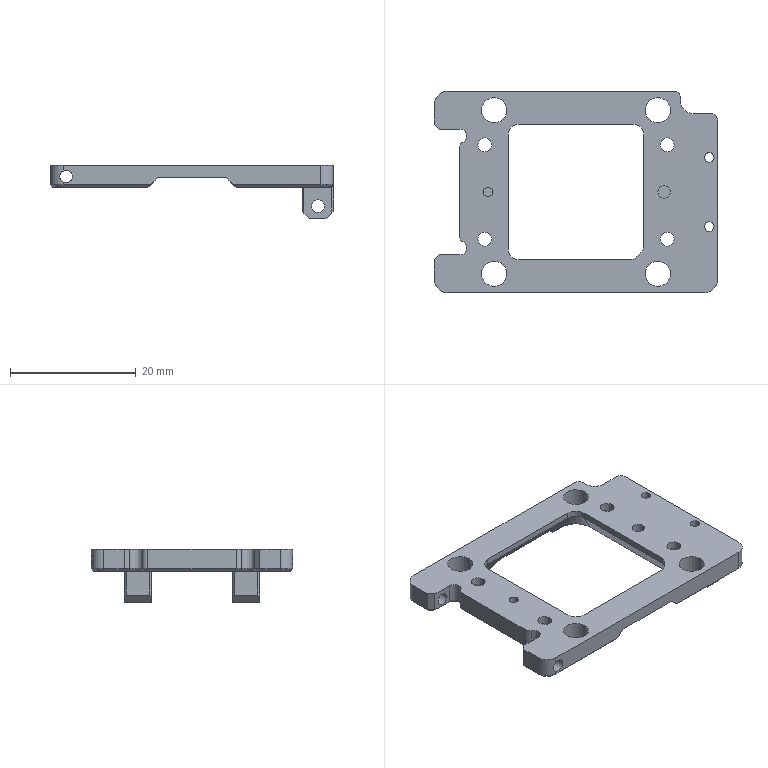NC program | NX | posted with a generic post | part box 45 x 32 x 8.5 mm
Lines 1818 to 2983 of 2983:
(ZLEVEL_PROFILE_1 , TOOL : D3R0.5)
N3592 T07 M6
N3594 G54
N3596 G17 G0 G90 X6.039 Y-10.352 B0. C0. S9500 M3
N3598 G43 Z30. H7
N3600 Z-3.587
N3602 G94 G1 Z-5.087 F1000.
N3604 X6.275 Y-10.756
N3606 G3 X6.536 Y-10.905 R0.3
N3608 G1 X8.847 Y-10.89 F2500.
N3610 G3 X9.951 Y-10.624 R2.492
N3612 X10.883 Y-9.005 R2.038
N3614 G1 X10.892 Y-8.762
N3616 X10.905 Y-5.354
N3618 X10.903 Y7.058
N3620 X10.89 Y8.886
N3622 G3 X10.466 Y10.153 R2.149
N3624 X9.005 Y10.883 R1.989
N3626 G1 X8.762 Y10.891
N3628 X6.571 Y10.904
N3630 X6.536 Y10.906
N3632 X6.444 Y10.858 Z-5.173
N3634 X6.571 Y10.854
N3636 X8.762 Y10.847
N3638 X9.005 Y10.839
N3640 G2 X10.763 Y9.483 R1.865
N3642 X10.848 Y8.88 R2.239
N3644 G1 X10.854 Y7.058
N3646 Y-7.058
N3648 X10.847 Y-8.762
N3650 G2 X10.827 Y-9.156 R3.694
N3652 X9.979 Y-10.559 R1.937
N3654 X8.881 Y-10.848 R2.251
N3656 G1 X6.571 Y-10.853
N3658 X6.444 Y-10.857
N3660 X6.351 Y-10.804 Z-5.26
N3662 X6.99 Y-10.805
N3664 X9.
N3666 G3 X10.045 Y-10.466 R2.012
N3668 X10.805 Y-9. R1.898
N3670 G1 Y9.
N3672 G3 X9. Y10.805 R1.841
N3674 G1 X6.99
N3676 X6.352
N3678 X6.26 Y10.757 Z-5.346
N3680 X6.328 Y10.754
N3682 X6.904 Y10.755
N3684 X9.
N3686 G2 X10.755 Y9. R1.755
N3688 G1 Y-9.
N3690 G2 X9. Y-10.755 R1.755
N3692 G1 X6.904
N3694 X6.328 Y-10.753
N3696 X6.259 Y-10.757
N3698 X6.167 Y-10.705 Z-5.433
N3700 X6.817
N3702 X9.
N3704 G3 X10.705 Y-9. R1.705
N3706 G1 Y9.
N3708 G3 X9. Y10.705 R1.705
N3710 G1 X6.817
N3712 X6.167 Y10.706
N3714 X6.075 Y10.655 Z-5.52
N3716 X6.73
N3718 X9.
N3720 G2 X10.655 Y9. R1.655
N3722 G1 Y-9.
N3724 G2 X9. Y-10.655 R1.655
N3726 G1 X6.73
N3728 X6.075
N3730 X5.983 Y-10.609 Z-5.606
N3732 X6.085 Y-10.604
N3734 X6.644 Y-10.605
N3736 X9.
N3738 G3 X10.605 Y-9. R1.605
N3740 G1 Y9.
N3742 G3 X9. Y10.605 R1.605
N3744 G1 X6.644
N3746 X6.085 Y10.604
N3748 X5.983 Y10.609
N3750 X5.891 Y10.558 Z-5.693
N3752 X6.557 Y10.555
N3754 X9.
N3756 G2 X10.555 Y9. R1.555
N3758 G1 Y-9.
N3760 G2 X9. Y-10.555 R1.555
N3762 G1 X6.557
N3764 X5.891 Y-10.558
N3766 X5.798 Y-10.507 Z-5.779
N3768 X5.841 Y-10.504
N3770 X6.471 Y-10.505
N3772 X9.
N3774 G3 X10.505 Y-9. R1.505
N3776 G1 Y9.
N3778 G3 X9. Y10.505 R1.505
N3780 G1 X6.471
N3782 X5.841
N3784 X5.798 Y10.507
N3786 X5.706 Y10.457 Z-5.866
N3788 X6.384 Y10.455
N3790 X9.
N3792 G2 X10.455 Y9. R1.455
N3794 G1 Y-9.
N3796 G2 X9. Y-10.455 R1.455
N3798 G1 X6.384
N3800 X5.841
N3802 X5.706 Y-10.457
N3804 X5.613 Y-10.405 Z-5.953
N3806 X6.297
N3808 X9.
N3810 G3 X10.405 Y-9. R1.405
N3812 G1 Y9.
N3814 G3 X9. Y10.405 R1.405
N3816 G1 X6.297
N3818 X5.613
N3820 X5.521 Y10.36 Z-6.039
N3822 X5.598 Y10.355
N3824 X6.211
N3826 X9.
N3828 G2 X10.355 Y9. R1.355
N3830 G1 Y-9.
N3832 G2 X9. Y-10.355 R1.355
N3834 G1 X6.211
N3836 X5.598
N3838 X5.521 Y-10.359
N3840 G2 X5.252 Y-10.226 R0.3
N3842 G1 X4.984 Y-9.822
N3844 Z-4.539
N3846 G0 Z30.
N3848 X4.93 Y-9.757
N3850 Z-4.626
N3852 G1 Z-6.126 F1000.
N3854 X5.168 Y-10.161
N3856 G3 X5.428 Y-10.309 R0.3
N3858 G1 X6.124 Y-10.305 F2500.
N3860 X9.
N3862 G3 X10.305 Y-9. R1.305
N3864 G1 Y9.
N3866 G3 X9. Y10.305 R1.305
N3868 G1 X6.124
N3870 X5.428 Y10.309
N3872 X5.336 Y10.256 Z-6.212
N3874 X6.038 Y10.255
N3876 X9.
N3878 G2 X10.255 Y9. R1.255
N3880 G1 Y-9.
N3882 G2 X9. Y-10.255 R1.255
N3884 G1 X6.038
N3886 X5.336 Y-10.256
N3888 X5.219 Y-10.257 Z-6.218
N3890 X5.102 Y-10.258 Z-6.223
N3892 X4.985 Y-10.254 Z-6.229
N3894 X4.868 Y-10.248 Z-6.234
N3896 X4.751 Y-10.245 Z-6.239
N3898 X4.634 Y-10.24 Z-6.245
N3900 X4.516 Y-10.236 Z-6.25
N3902 X4.399 Y-10.232 Z-6.256
N3904 X4.282 Y-10.229 Z-6.261
N3906 X4.165 Y-10.225 Z-6.267
N3908 X4.048 Y-10.221 Z-6.272
N3910 X3.931 Y-10.218 Z-6.277
N3912 X3.814 Y-10.214 Z-6.283
N3914 X3.697 Y-10.211 Z-6.288
N3916 X3.58 Y-10.208 Z-6.294
N3918 X3.463 Y-10.205 Z-6.299
N3920 X5.951
N3922 X9.
N3924 G3 X10.205 Y-9. R1.205
N3926 G1 Y9.
N3928 G3 X9. Y10.205 R1.205
N3930 G1 X5.951
N3932 X3.497
N3934 G3 X3.237 Y10.055 R0.3
N3936 G1 X2.978 Y9.605
N3938 Z-4.799
N3940 G0 Z30.
N3942 X-6.039 Y10.352
N3944 Z-3.587
N3946 G1 Z-5.087 F1000.
N3948 X-6.275 Y10.756
N3950 G3 X-6.536 Y10.905 R0.3
N3952 G1 X-8.762 Y10.89 F2500.
N3954 X-9.005 Y10.882
N3956 G3 X-10.466 Y10.153 R1.983
N3958 X-10.892 Y8.88 R2.18
N3960 G1 X-10.903 Y7.788
N3962 Y-6.815
N3964 X-10.893 Y-8.114
N3966 G3 X-10.827 Y-8.762 R3.463
N3968 X-10.311 Y-9.735 R2.099
N3970 G1 X-9.829 Y-10.222
N3972 X-9.697 Y-10.342
N3974 G3 X-8.657 Y-10.844 R1.994
N3976 X-8.275 Y-10.891 R6.142
N3978 G1 X-6.536 Y-10.906
N3980 X-6.444 Y-10.858 Z-5.173
N3982 X-6.571 Y-10.853
N3984 X-8.275 Y-10.847
N3986 G2 X-9.249 Y-10.609 R2.255
N3988 X-10.008 Y-9.979 R3.046
N3990 X-10.609 Y-9.249 R2.964
N3992 X-10.847 Y-8.275 R2.214
N3994 G1 X-10.854 Y-6.815
N3996 X-10.855 Y4.381
N3998 X-10.848 Y8.762
N4000 X-10.84 Y9.005
N4002 G2 X-9.005 Y10.841 R1.879
N4004 G1 X-8.762 Y10.848
N4006 X-6.571 Y10.853
N4008 X-6.444 Y10.857
N4010 X-6.352 Y10.804 Z-5.26
N4012 X-6.99 Y10.805
N4014 X-9.
N4016 G3 X-10.805 Y9. R1.841
N4018 G1 Y-8.275
N4020 G3 X-10.709 Y-8.929 R2.675
N4022 X-10.222 Y-9.709 R2.104
N4024 G1 X-9.709 Y-10.222
N4026 G3 X-8.929 Y-10.709 R2.066
N4028 X-8.275 Y-10.805 R2.735
N4030 G1 X-6.99
N4032 X-6.352
N4034 X-6.259 Y-10.757 Z-5.346
N4036 X-6.328 Y-10.754
N4038 X-6.904 Y-10.755
N4040 X-8.379
N4042 G2 X-9.619 Y-10.241 R1.755
N4044 G1 X-10.241 Y-9.619
N4046 G2 X-10.755 Y-8.379 R1.755
N4048 G1 Y9.
N4050 G2 X-9. Y10.755 R1.755
N4052 G1 X-6.904
N4054 X-6.328 Y10.753
N4056 X-6.26 Y10.757
N4058 X-6.167 Y10.705 Z-5.433
N4060 X-6.817
N4062 X-9.
N4064 G3 X-10.705 Y9. R1.705
N4066 G1 Y-8.379
N4068 G3 X-10.205 Y-9.584 R1.705
N4070 G1 X-9.584 Y-10.205
N4072 G3 X-8.379 Y-10.705 R1.705
N4074 G1 X-6.817
N4076 X-6.167
N4078 X-6.075 Y-10.655 Z-5.52
N4080 X-6.73
N4082 X-8.379
N4084 G2 X-9.549 Y-10.17 R1.655
N4086 G1 X-10.17 Y-9.549
N4088 G2 X-10.655 Y-8.379 R1.655
N4090 G1 Y9.
N4092 G2 X-9. Y10.655 R1.655
N4094 G1 X-6.73
N4096 X-6.075
N4098 X-5.983 Y10.609 Z-5.606
N4100 X-6.085 Y10.604
N4102 X-6.644 Y10.605
N4104 X-9.
N4106 G3 X-10.605 Y9. R1.605
N4108 G1 Y-8.379
N4110 G3 X-10.135 Y-9.513 R1.605
N4112 G1 X-9.513 Y-10.135
N4114 G3 X-8.379 Y-10.605 R1.605
N4116 G1 X-6.644
N4118 X-6.085 Y-10.604
N4120 X-5.983 Y-10.609
N4122 X-5.891 Y-10.558 Z-5.693
N4124 X-6.557 Y-10.555
N4126 X-8.379
N4128 G2 X-9.478 Y-10.099 R1.555
N4130 G1 X-10.099 Y-9.478
N4132 G2 X-10.555 Y-8.379 R1.555
N4134 G1 Y9.
N4136 G2 X-9. Y10.555 R1.555
N4138 G1 X-6.557
N4140 X-5.891 Y10.558
N4142 X-5.799 Y10.507 Z-5.779
N4144 X-5.841 Y10.505
N4146 X-6.471
N4148 X-9.
N4150 G3 X-10.505 Y9. R1.505
N4152 G1 Y-8.379
N4154 G3 X-10.064 Y-9.443 R1.505
N4156 G1 X-9.443 Y-10.064
N4158 G3 X-8.379 Y-10.505 R1.505
N4160 G1 X-6.471
N4162 X-5.841
N4164 X-5.798 Y-10.507
N4166 X-5.706 Y-10.457 Z-5.866
N4168 X-5.841 Y-10.455
N4170 X-6.384
N4172 X-8.379
N4174 G2 X-9.407 Y-10.029 R1.455
N4176 G1 X-10.029 Y-9.407
N4178 G2 X-10.455 Y-8.379 R1.455
N4180 G1 Y9.
N4182 G2 X-9. Y10.455 R1.455
N4184 G1 X-6.384
N4186 X-5.841
N4188 X-5.706 Y10.457
N4190 X-5.613 Y10.405 Z-5.953
N4192 X-6.297
N4194 X-9.
N4196 G3 X-10.405 Y9. R1.405
N4198 G1 Y-8.379
N4200 G3 X-9.993 Y-9.372 R1.405
N4202 G1 X-9.372 Y-9.993
N4204 G3 X-8.379 Y-10.405 R1.405
N4206 G1 X-6.297
N4208 X-5.613
N4210 X-5.521 Y-10.359 Z-6.039
N4212 X-5.598 Y-10.355
N4214 X-6.211
N4216 X-8.379
N4218 G2 X-9.337 Y-9.958 R1.355
N4220 G1 X-9.958 Y-9.337
N4222 G2 X-10.355 Y-8.379 R1.355
N4224 G1 Y9.
N4226 G2 X-9. Y10.355 R1.355
N4228 G1 X-6.211
N4230 X-5.598
N4232 X-5.521 Y10.359
N4234 G2 X-5.252 Y10.226 R0.3
N4236 G1 X-4.984 Y9.822
N4238 Z-4.539
N4240 G0 Z30.
N4242 X-4.93 Y9.757
N4244 Z-4.626
N4246 G1 Z-6.126 F1000.
N4248 X-5.167 Y10.161
N4250 G3 X-5.428 Y10.309 R0.3
N4252 G1 X-6.124 Y10.305 F2500.
N4254 X-9.
N4256 G3 X-10.305 Y9. R1.305
N4258 G1 Y-8.379
N4260 G3 X-9.923 Y-9.301 R1.305
N4262 G1 X-9.301 Y-9.923
N4264 G3 X-8.379 Y-10.305 R1.305
N4266 G1 X-6.124
N4268 X-5.428 Y-10.309
N4270 X-5.336 Y-10.256 Z-6.212
N4272 X-6.038 Y-10.255
N4274 X-8.379
N4276 G2 X-9.266 Y-9.887 R1.255
N4278 G1 X-9.887 Y-9.266
N4280 G2 X-10.255 Y-8.379 R1.255
N4282 G1 Y9.
N4284 G2 X-9. Y10.255 R1.255
N4286 G1 X-6.038
N4288 X-5.336 Y10.256
N4290 X-5.221 Y10.257 Z-6.218
N4292 X-5.106 Y10.258 Z-6.223
N4294 X-4.991 Y10.254 Z-6.229
N4296 X-4.876 Y10.248 Z-6.234
N4298 X-4.761 Y10.245 Z-6.239
N4300 X-4.646 Y10.24 Z-6.245
N4302 X-4.531 Y10.236 Z-6.25
N4304 X-4.416 Y10.232 Z-6.256
N4306 X-4.301 Y10.229 Z-6.261
N4308 X-4.186 Y10.225 Z-6.267
N4310 X-4.071 Y10.221 Z-6.272
N4312 X-3.956 Y10.218 Z-6.277
N4314 X-3.841 Y10.215 Z-6.283
N4316 X-3.726 Y10.211 Z-6.288
N4318 X-3.611 Y10.208 Z-6.294
N4320 X-3.497 Y10.205 Z-6.299
N4322 X-5.951
N4324 X-9.
N4326 G3 X-10.205 Y9. R1.205
N4328 G1 Y-8.379
N4330 G3 X-9.852 Y-9.231 R1.205
N4332 G1 X-9.231 Y-9.852
N4334 G3 X-8.379 Y-10.205 R1.205
N4336 G1 X-5.951
N4338 X-3.462
N4340 G3 X-3.202 Y-10.055 R0.3
N4342 G1 X-2.942 Y-9.605
N4344 Z-4.799
N4346 G0 Z30.
N4348 X-0.52 Y9.555
N4350 Z-4.886
N4352 G1 Z-6.386 F1000.
N4354 X-0.26 Y10.005
N4356 G2 X0. Y10.155 R0.3
N4358 G1 X9. F2500.
N4360 G2 X10.155 Y9. R1.155
N4362 G1 Y-9.
N4364 G2 X9. Y-10.155 R1.155
N4366 G1 X-8.379
N4368 G2 X-9.195 Y-9.816 R1.155
N4370 G1 X-9.816 Y-9.195
N4372 G2 X-10.155 Y-8.379 R1.155
N4374 G1 Y9.
N4376 G2 X-9. Y10.155 R1.155
N4378 G1 X0.
N4380 Y10.13 Z-6.429
N4382 Y10.105 Z-6.472
N4384 X-9.
N4386 G3 X-10.105 Y9. R1.105
N4388 G1 Y-8.379
N4390 G3 X-9.781 Y-9.16 R1.105
N4392 G1 X-9.16 Y-9.781
N4394 G3 X-8.379 Y-10.105 R1.105
N4396 G1 X9.
N4398 G3 X10.105 Y-9. R1.105
N4400 G1 Y9.
N4402 G3 X9. Y10.105 R1.105
N4404 G1 X0.
N4406 Y10.08 Z-6.516
N4408 Y10.055 Z-6.559
N4410 X9.
N4412 G2 X10.055 Y9. R1.055
N4414 G1 Y-9.
N4416 G2 X9. Y-10.055 R1.055
N4418 G1 X-8.379
N4420 G2 X-9.124 Y-9.746 R1.055
N4422 G1 X-9.746 Y-9.124
N4424 G2 X-10.055 Y-8.379 R1.055
N4426 G1 Y9.
N4428 G2 X-9. Y10.055 R1.055
N4430 G1 X0.
N4432 Y10.03 Z-6.602
N4434 Y10.005 Z-6.645
N4436 X-9.
N4438 G3 X-10.005 Y9. R1.005
N4440 G1 Y-8.379
N4442 G3 X-9.71 Y-9.089 R1.005
N4444 G1 X-9.089 Y-9.71
N4446 G3 X-8.379 Y-10.005 R1.005
N4448 G1 X9.
N4450 G3 X10.005 Y-9. R1.005
N4452 G1 Y9.
N4454 G3 X9. Y10.005 R1.005
N4456 G1 X0.
N4458 Y9.955 Z-6.732
N4460 X9.
N4462 G2 X9.955 Y9. R0.955
N4464 G1 Y-9.
N4466 G2 X9. Y-9.955 R0.955
N4468 G1 X-8.379
N4470 G2 X-9.054 Y-9.675 R0.955
N4472 G1 X-9.675 Y-9.054
N4474 G2 X-9.955 Y-8.379 R0.955
N4476 G1 Y9.
N4478 G2 X-9. Y9.955 R0.955
N4480 G1 X0.
N4482 Y9.905 Z-6.819
N4484 X-9.
N4486 G3 X-9.905 Y9. R0.905
N4488 G1 Y-8.379
N4490 G3 X-9.64 Y-9.018 R0.905
N4492 G1 X-9.018 Y-9.64
N4494 G3 X-8.379 Y-9.905 R0.905
N4496 G1 X9.
N4498 G3 X9.905 Y-9. R0.905
N4500 G1 Y9.
N4502 G3 X9. Y9.905 R0.905
N4504 G1 X0.
N4506 Y9.855 Z-6.905
N4508 X9.
N4510 G2 X9.855 Y9. R0.855
N4512 G1 Y-9.
N4514 G2 X9. Y-9.855 R0.855
N4516 G1 X-8.379
N4518 G2 X-8.983 Y-9.604 R0.855
N4520 G1 X-9.604 Y-8.983
N4522 G2 X-9.855 Y-8.379 R0.855
N4524 G1 Y9.
N4526 G2 X-9. Y9.855 R0.855
N4528 G1 X0.
N4530 Y9.805 Z-6.992
N4532 X-9.
N4534 G3 X-9.805 Y9. R0.805
N4536 G1 Y-8.379
N4538 G3 X-9.569 Y-8.948 R0.805
N4540 G1 X-8.948 Y-9.569
N4542 G3 X-8.379 Y-9.805 R0.805
N4544 G1 X9.
N4546 G3 X9.805 Y-9. R0.805
N4548 G1 Y9.
N4550 G3 X9. Y9.805 R0.805
N4552 G1 X0.
N4554 Y9.755 Z-7.078
N4556 X9.
N4558 G2 X9.755 Y9. R0.755
N4560 G1 Y-9.
N4562 G2 X9. Y-9.755 R0.755
N4564 G1 X-8.379
N4566 G2 X-8.912 Y-9.534 R0.755
N4568 G1 X-9.534 Y-8.912
N4570 G2 X-9.755 Y-8.379 R0.755
N4572 G1 Y9.
N4574 G2 X-9. Y9.755 R0.755
N4576 G1 X0.
N4578 Y9.705 Z-7.165
N4580 X-9.
N4582 G3 X-9.705 Y9. R0.705
N4584 G1 Y-8.379
N4586 G3 X-9.498 Y-8.877 R0.705
N4588 G1 X-8.877 Y-9.498
N4590 G3 X-8.379 Y-9.705 R0.705
N4592 G1 X9.
N4594 G3 X9.705 Y-9. R0.705
N4596 G1 Y9.
N4598 G3 X9. Y9.705 R0.705
N4600 G1 X0.
N4602 Y9.655 Z-7.252
N4604 X9.
N4606 G2 X9.655 Y9. R0.655
N4608 G1 Y-9.
N4610 G2 X9. Y-9.655 R0.655
N4612 G1 X-8.379
N4614 G2 X-8.842 Y-9.463 R0.655
N4616 G1 X-9.463 Y-8.842
N4618 G2 X-9.655 Y-8.379 R0.655
N4620 G1 Y9.
N4622 G2 X-9. Y9.655 R0.655
N4624 G1 X0.
N4626 Y9.605 Z-7.338
N4628 X-9.
N4630 G3 X-9.605 Y9. R0.605
N4632 G1 Y-8.379
N4634 G3 X-9.428 Y-8.806 R0.605
N4636 G1 X-8.806 Y-9.428
N4638 G3 X-8.379 Y-9.605 R0.605
N4640 G1 X9.
N4642 G3 X9.605 Y-9. R0.605
N4644 G1 Y9.
N4646 G3 X9. Y9.605 R0.605
N4648 G1 X0.
N4650 Y9.555 Z-7.425
N4652 X9.
N4654 G2 X9.555 Y9. R0.555
N4656 G1 Y-9.
N4658 G2 X9. Y-9.555 R0.555
N4660 G1 X-8.379
N4662 G2 X-8.771 Y-9.392 R0.555
N4664 G1 X-9.392 Y-8.771
N4666 G2 X-9.555 Y-8.379 R0.555
N4668 G1 Y9.
N4670 G2 X-9. Y9.555 R0.555
N4672 G1 X0.
N4674 Y9.505 Z-7.511
N4676 X-9.
N4678 G3 X-9.505 Y9. R0.505
N4680 G1 Y-8.379
N4682 G3 X-9.357 Y-8.736 R0.505
N4684 G1 X-8.736 Y-9.357
N4686 G3 X-8.379 Y-9.505 R0.505
N4688 G1 X9.
N4690 G3 X9.505 Y-9. R0.505
N4692 G1 Y9.
N4694 G3 X9. Y9.505 R0.505
N4696 G1 X0.
N4698 Y9.455 Z-7.598
N4700 X9.
N4702 G2 X9.455 Y9. R0.455
N4704 G1 Y-9.
N4706 G2 X9. Y-9.455 R0.455
N4708 G1 X-8.379
N4710 G2 X-8.7 Y-9.322 R0.455
N4712 G1 X-9.322 Y-8.7
N4714 G2 X-9.455 Y-8.379 R0.455
N4716 G1 Y9.
N4718 G2 X-9. Y9.455 R0.455
N4720 G1 X0.
N4722 Y9.405 Z-7.685
N4724 X-9.
N4726 G3 X-9.405 Y9. R0.405
N4728 G1 Y-8.379
N4730 G3 X-9.286 Y-8.665 R0.405
N4732 G1 X-8.665 Y-9.286
N4734 G3 X-8.379 Y-9.405 R0.405
N4736 G1 X9.
N4738 G3 X9.405 Y-9. R0.405
N4740 G1 Y9.
N4742 G3 X9. Y9.405 R0.405
N4744 G1 X0.
N4746 Y9.382 Z-7.724
N4748 Y9.359 Z-7.764
N4750 X8.762
N4752 X9.005 Y9.354
N4754 G2 X9.354 Y9.005 R0.349
N4756 G1 X9.359 Y8.762
N4758 Y-8.762
N4760 X9.354 Y-9.005
N4762 G2 X9.005 Y-9.354 R0.35
N4764 G1 X8.762 Y-9.359
N4766 X-8.369
N4768 G2 X-8.629 Y-9.251 R0.368
N4770 G1 X-9.249 Y-8.631
N4772 G2 X-9.353 Y-8.397 R0.311
N4774 G1 X-9.359 Y-8.275
N4776 Y8.762
N4778 X-9.354 Y9.005
N4780 G2 X-9.005 Y9.354 R0.349
N4782 G1 X-8.762 Y9.359
N4784 X0.
N4786 Y9.336 Z-7.803
N4788 Y9.312 Z-7.842
N4790 X-8.762
N4792 X-9.005 Y9.307
N4794 G3 X-9.306 Y9.005 R0.304
N4796 G1 X-9.312 Y8.762
N4798 Y-8.275
N4800 X-9.306 Y-8.397
N4802 X-9.31 Y-8.457
N4804 X-9.289 Y-8.513
N4806 X-9.249 Y-8.557
N4808 G3 X-8.578 Y-9.23 R10.038
N4810 X-8.366 Y-9.312 R0.314
N4812 G1 X8.762
N4814 X9.005 Y-9.307
N4816 G3 X9.307 Y-9.005 R0.304
N4818 G1 X9.312 Y-8.762
N4820 Y8.762
N4822 X9.307 Y9.005
N4824 G3 X9.005 Y9.306 R0.304
N4826 G1 X8.762 Y9.312
N4828 X0.
N4830 Y9.291 Z-7.882
N4832 Y9.265 Z-7.921
N4834 X8.762
N4836 X9.005 Y9.259
N4838 G2 X9.26 Y9.005 R0.253
N4840 G1 X9.264 Y8.762
N4842 X9.265 Y-8.762
N4844 X9.259 Y-9.005
N4846 G2 X9.005 Y-9.26 R0.254
N4848 G1 X8.762 Y-9.264
N4850 X-8.275
N4852 X-8.397 Y-9.259
N4854 X-8.442 Y-9.265
N4856 X-8.486 Y-9.251
N4858 X-8.518 Y-9.219
N4860 G2 X-9.22 Y-8.518 R9.913
N4862 G1 X-9.251 Y-8.485
N4864 X-9.265 Y-8.442
N4866 X-9.259 Y-8.397
N4868 X-9.264 Y-8.275
N4870 X-9.265 Y8.762
N4872 X-9.259 Y9.005
N4874 G2 X-9.005 Y9.26 R0.254
N4876 G1 X-8.762 Y9.264
N4878 X0. Y9.265
N4880 Y9.245 Z-7.961
N4882 Y9.218 Z-8.
N4884 X-8.762
N4886 X-9.005 Y9.213
N4888 G3 X-9.213 Y9.005 R0.211
N4890 G1 X-9.218 Y8.762
N4892 Y-8.275
N4894 X-9.212 Y-8.416
N4896 Y-8.463
N4898 X-9.179 Y-8.496
N4900 G3 X-8.504 Y-9.172 R9.98
N4902 G1 X-8.464 Y-9.21
N4904 X-8.409 Y-9.212
N4906 X-8.275 Y-9.218
N4908 X8.762
N4910 X9.005 Y-9.214
N4912 G3 X9.213 Y-9.005 R0.211
N4914 G1 X9.218 Y-8.762
N4916 Y8.762
N4918 X9.214 Y9.005
N4920 G3 X9.005 Y9.213 R0.21
N4922 G1 X8.762 Y9.218
N4924 X0.
N4926 G3 X-0.26 Y9.068 R0.3
N4928 G1 X-0.52 Y8.618
N4930 Z-6.5
N4932 G0 Z30.
(ZLEVEL_PROFILE_1_COPY , TOOL : D3R0.5)
N4934 X-5.195 Y16.634
N4936 Z-3.571
N4938 G1 Z-5.071 F1000.
N4940 X-5.594 Y16.362
N4942 G3 X-5.724 Y16.092 R0.3
N4944 G1 X-5.722 Y16.071 F2500.
N4946 Y11.936
N4948 X-5.724 Y11.782
N4950 X-5.653 Y11.74 Z-5.141
N4952 X-5.651 Y11.936
N4954 Y16.071
N4956 X-5.656 Y16.162
N4958 X-5.584 Y16.232 Z-5.212
N4960 X-5.581 Y15.666
N4962 Y12.205
N4964 Y11.699
N4966 X-5.512 Y11.658 Z-5.283
N4968 X-5.51 Y11.693
N4970 Y15.736
N4972 Y16.303
N4974 X-5.442 Y16.356 Z-5.354
N4976 X-5.439 Y16.314
N4978 Y11.693
N4980 X-5.443 Y11.616
N4982 X-5.372 Y11.575 Z-5.424
N4984 X-5.369 Y12.083
N4986 Y16.314
N4988 X-5.372 Y16.406
N4990 X-5.3 Y16.456 Z-5.495
N4992 X-5.298 Y15.949
N4994 Y12.042
N4996 X-5.3 Y11.534
N4998 X-5.228 Y11.492 Z-5.566
N5000 X-5.227 Y12.001
N5002 Y16.
N5004 X-5.229 Y16.462
N5006 X-5.192 Y16.463 Z-5.601
N5008 X-5.159 Z-5.636
N5010 X-5.156 Y16.
N5012 Y11.96
N5014 X-5.157 Y11.451
N5016 X-5.088 Y11.41 Z-5.707
N5018 X-5.086 Y11.45
N5020 Y16.071
N5022 X-5.088 Y16.463
N5024 X-5.05 Y16.464 Z-5.742
N5026 X-5.017 Z-5.778
N5028 X-5.015 Y16.071
N5030 Y11.45
N5032 X-5.018 Y11.368
N5034 X-4.948 Y11.327 Z-5.849
N5036 X-4.944 Y11.838
N5038 Y16.071
N5040 X-4.946 Y16.464
N5042 X-4.909 Y16.465 Z-5.884
N5044 X-4.876 Z-5.919
N5046 X-4.874 Y16.071
N5048 Y11.797
N5050 X-4.876 Y11.286
N5052 X-4.803 Y11.245 Z-5.99
N5054 Y11.756
N5056 Y16.071
N5058 X-4.805 Y16.465
N5060 X-4.768 Y16.466 Z-6.025
N5062 X-4.734 Z-6.061
N5064 X-4.732 Y16.071
N5066 Y11.716
N5068 Y11.204
N5070 X-4.664 Y11.163 Z-6.131
N5072 X-4.662 Y11.206
N5074 Y16.071
N5076 X-4.663 Y16.466
N5078 X-4.626 Y16.467 Z-6.167
N5080 X-4.593 Z-6.202
N5082 X-4.591 Y16.071
N5084 Y11.206
N5086 X-4.594 Y11.122
N5088 X-4.523 Y11.08 Z-6.273
N5090 X-4.52 Y11.593
N5092 Y16.071
N5094 X-4.522 Y16.467
N5096 X-4.492 Y16.468 Z-6.301
N5098 X-4.465 Z-6.33
N5100 X-4.463 Y16.071
N5102 Y11.56
N5104 X-4.466 Y11.047
N5106 X-4.408 Y11.014 Z-6.386
N5108 X-4.406 Y11.527
N5110 Y16.071
N5112 X-4.408 Y16.468
N5114 X-4.378 Z-6.415
N5116 X-4.352 Z-6.443
N5118 X-4.35 Y16.
N5120 Y11.495
N5122 Y10.981
N5124 X-4.295 Y10.963 Z-6.5
N5126 Y11.463
N5128 Y16.
N5130 Y16.325
N5132 G2 X-4.145 Y16.584 R0.3
N5134 G1 X-3.727 Y16.826
N5136 Z-5.
N5138 G0 Z30.
N5140 X5.186 Y11.285
N5142 Z-3.571
N5144 G1 Z-5.071 F1000.
N5146 X5.578 Y11.52
N5148 G3 X5.724 Y11.782 R0.3
N5150 G1 X5.722 Y11.936 F2500.
N5152 Y16.071
N5154 X5.724 Y16.092
N5156 X5.656 Y16.162 Z-5.141
N5158 X5.651 Y16.071
N5160 Y11.936
N5162 X5.653 Y11.74
N5164 X5.581 Y11.699 Z-5.212
N5166 Y12.205
N5168 Y15.666
N5170 X5.584 Y16.232
N5172 X5.51 Y16.303 Z-5.283
N5174 Y15.736
N5176 Y11.693
N5178 X5.512 Y11.658
N5180 X5.443 Y11.616 Z-5.354
N5182 X5.439 Y11.693
N5184 Y16.314
N5186 X5.442 Y16.356
N5188 X5.372 Y16.406 Z-5.424
N5190 X5.369 Y16.314
N5192 Y12.083
N5194 X5.372 Y11.575
N5196 X5.3 Y11.534 Z-5.495
N5198 X5.298 Y12.042
N5200 Y15.949
N5202 X5.3 Y16.456
N5204 X5.263 Y16.46 Z-5.53
N5206 X5.229 Y16.462 Z-5.566
N5208 X5.227 Y16.
N5210 Y12.001
N5212 X5.228 Y11.492
N5214 X5.157 Y11.451 Z-5.636
N5216 X5.156 Y11.96
N5218 Y16.
N5220 X5.159 Y16.463
N5222 X5.121 Z-5.672
N5224 X5.088 Z-5.707
N5226 X5.086 Y16.071
N5228 Y11.45
N5230 X5.088 Y11.41
N5232 X5.018 Y11.368 Z-5.778
N5234 X5.015 Y11.45
N5236 Y16.071
N5238 X5.017 Y16.464
N5240 X4.98 Z-5.813
N5242 X4.946 Z-5.849
N5244 X4.944 Y16.071
N5246 Y11.838
N5248 X4.948 Y11.327
N5250 X4.876 Y11.286 Z-5.919
N5252 X4.874 Y11.797
N5254 Y16.071
N5256 X4.876 Y16.465
N5258 X4.838 Z-5.955
N5260 X4.805 Z-5.99
N5262 X4.803 Y16.071
N5264 Y11.756
N5266 Y11.245
N5268 X4.732 Y11.204 Z-6.061
N5270 Y11.716
N5272 Y16.071
N5274 X4.734 Y16.466
N5276 X4.697 Z-6.096
N5278 X4.663 Z-6.131
N5280 X4.662 Y16.071
N5282 Y11.206
N5284 X4.664 Y11.163
N5286 X4.594 Y11.122 Z-6.202
N5288 X4.591 Y11.206
N5290 Y16.071
N5292 X4.593 Y16.467
N5294 X4.555 Z-6.237
N5296 X4.522 Z-6.273
N5298 X4.52 Y16.071
N5300 Y11.593
N5302 X4.523 Y11.08
N5304 X4.466 Y11.047 Z-6.33
N5306 X4.463 Y11.56
N5308 Y16.071
N5310 X4.465 Y16.468
N5312 X4.435 Z-6.358
N5314 X4.408 Z-6.386
N5316 X4.406 Y16.071
N5318 Y11.527
N5320 X4.408 Y11.014
N5322 X4.35 Y10.981 Z-6.443
N5324 Y11.495
N5326 Y16.
N5328 X4.352 Y16.468
N5330 X4.321 Y16.397 Z-6.472
N5332 X4.295 Y16.325 Z-6.5
N5334 Y16.
N5336 Y11.463
N5338 X4.285 Y11.45
N5340 X4.295 Y10.963
N5342 G2 X4.15 Y10.7 R0.3
N5344 G1 X3.756 Y10.462
N5346 Z-5.
N5348 G0 Z30.
N5350 X5.195 Y-16.634
N5352 Z-3.571
N5354 G1 Z-5.071 F1000.
N5356 X5.594 Y-16.362
N5358 G3 X5.724 Y-16.092 R0.3
N5360 G1 X5.722 Y-16.071 F2500.
N5362 Y-11.936
N5364 X5.724 Y-11.782
N5366 X5.653 Y-11.74 Z-5.141
N5368 X5.651 Y-11.936
N5370 Y-16.071
N5372 X5.656 Y-16.162
N5374 X5.584 Y-16.232 Z-5.212
N5376 X5.581 Y-15.666
N5378 Y-12.205
N5380 Y-11.699
N5382 X5.512 Y-11.658 Z-5.283
N5384 X5.51 Y-11.693
N5386 Y-15.736
N5388 Y-16.303
N5390 X5.442 Y-16.356 Z-5.354
N5392 X5.439 Y-16.314
N5394 Y-11.693
N5396 X5.443 Y-11.616
N5398 X5.372 Y-11.575 Z-5.424
N5400 X5.369 Y-12.083
N5402 Y-16.314
N5404 X5.372 Y-16.406
N5406 X5.3 Y-16.456 Z-5.495
N5408 X5.298 Y-15.949
N5410 Y-12.042
N5412 X5.3 Y-11.534
N5414 X5.228 Y-11.492 Z-5.566
N5416 X5.227 Y-12.001
N5418 Y-16.
N5420 X5.229 Y-16.462
N5422 X5.192 Y-16.463 Z-5.601
N5424 X5.159 Z-5.636
N5426 X5.156 Y-16.
N5428 Y-11.96
N5430 X5.157 Y-11.451
N5432 X5.088 Y-11.41 Z-5.707
N5434 X5.086 Y-11.45
N5436 Y-16.071
N5438 X5.088 Y-16.463
N5440 X5.05 Y-16.464 Z-5.742
N5442 X5.017 Z-5.778
N5444 X5.015 Y-16.071
N5446 Y-11.45
N5448 X5.018 Y-11.369
N5450 X4.948 Y-11.327 Z-5.849
N5452 X4.944 Y-11.838
N5454 Y-16.071
N5456 X4.946 Y-16.464
N5458 X4.909 Y-16.465 Z-5.884
N5460 X4.876 Z-5.919
N5462 X4.874 Y-16.071
N5464 Y-11.797
N5466 X4.876 Y-11.286
N5468 X4.803 Y-11.245 Z-5.99
N5470 Y-11.756
N5472 Y-16.071
N5474 X4.805 Y-16.465
N5476 X4.768 Y-16.466 Z-6.025
N5478 X4.734 Z-6.061
N5480 X4.732 Y-16.071
N5482 Y-11.716
N5484 Y-11.204
N5486 X4.664 Y-11.163 Z-6.131
N5488 X4.662 Y-11.206
N5490 Y-16.071
N5492 X4.663 Y-16.466
N5494 X4.626 Y-16.467 Z-6.167
N5496 X4.593 Z-6.202
N5498 X4.591 Y-16.071
N5500 Y-11.206
N5502 X4.594 Y-11.121
N5504 X4.523 Y-11.08 Z-6.273
N5506 X4.52 Y-11.593
N5508 Y-16.071
N5510 X4.522 Y-16.467
N5512 X4.492 Y-16.468 Z-6.301
N5514 X4.465 Z-6.33
N5516 X4.463 Y-16.071
N5518 Y-11.56
N5520 X4.466 Y-11.047
N5522 X4.408 Y-11.014 Z-6.386
N5524 X4.406 Y-11.527
N5526 Y-16.071
N5528 X4.408 Y-16.468
N5530 X4.378 Z-6.415
N5532 X4.352 Y-16.469 Z-6.443
N5534 X4.35 Y-16.
N5536 Y-11.495
N5538 Y-10.981
N5540 X4.295 Y-10.963 Z-6.5
N5542 X4.285 Y-11.45
N5544 X4.295 Y-11.463
N5546 Y-16.
N5548 Y-16.325
N5550 G2 X4.145 Y-16.584 R0.3
N5552 G1 X3.728 Y-16.825
N5554 Z-5.
N5556 G0 Z30.
N5558 X-5.186 Y-11.285
N5560 Z-3.571
N5562 G1 Z-5.071 F1000.
N5564 X-5.578 Y-11.52
N5566 G3 X-5.724 Y-11.782 R0.3
N5568 G1 X-5.722 Y-11.936 F2500.
N5570 Y-16.071
N5572 X-5.724 Y-16.092
N5574 X-5.656 Y-16.162 Z-5.141
N5576 X-5.651 Y-16.071
N5578 Y-11.936
N5580 X-5.653 Y-11.74
N5582 X-5.581 Y-11.699 Z-5.212
N5584 Y-12.205
N5586 Y-15.666
N5588 X-5.584 Y-16.232
N5590 X-5.51 Y-16.303 Z-5.283
N5592 Y-15.736
N5594 Y-11.693
N5596 X-5.512 Y-11.658
N5598 X-5.443 Y-11.616 Z-5.354
N5600 X-5.439 Y-11.693
N5602 Y-16.314
N5604 X-5.442 Y-16.356
N5606 X-5.372 Y-16.406 Z-5.424
N5608 X-5.369 Y-16.314
N5610 Y-12.083
N5612 X-5.372 Y-11.575
N5614 X-5.3 Y-11.534 Z-5.495
N5616 X-5.298 Y-12.042
N5618 Y-15.949
N5620 X-5.3 Y-16.456
N5622 X-5.263 Y-16.46 Z-5.53
N5624 X-5.229 Y-16.462 Z-5.566
N5626 X-5.227 Y-16.
N5628 Y-12.001
N5630 X-5.228 Y-11.492
N5632 X-5.157 Y-11.451 Z-5.636
N5634 X-5.156 Y-11.96
N5636 Y-16.
N5638 X-5.159 Y-16.463
N5640 X-5.121 Z-5.672
N5642 X-5.088 Z-5.707
N5644 X-5.086 Y-16.071
N5646 Y-11.45
N5648 X-5.088 Y-11.41
N5650 X-5.018 Y-11.369 Z-5.778
N5652 X-5.015 Y-11.45
N5654 Y-16.071
N5656 X-5.017 Y-16.464
N5658 X-4.98 Z-5.813
N5660 X-4.946 Z-5.849
N5662 X-4.944 Y-16.071
N5664 Y-11.838
N5666 X-4.948 Y-11.327
N5668 X-4.876 Y-11.286 Z-5.919
N5670 X-4.874 Y-11.797
N5672 Y-16.071
N5674 X-4.876 Y-16.465
N5676 X-4.838 Z-5.955
N5678 X-4.805 Z-5.99
N5680 X-4.803 Y-16.071
N5682 Y-11.756
N5684 Y-11.245
N5686 X-4.732 Y-11.204 Z-6.061
N5688 Y-11.716
N5690 Y-16.071
N5692 X-4.734 Y-16.466
N5694 X-4.697 Z-6.096
N5696 X-4.663 Z-6.131
N5698 X-4.662 Y-16.071
N5700 Y-11.206
N5702 X-4.664 Y-11.163
N5704 X-4.594 Y-11.121 Z-6.202
N5706 X-4.591 Y-11.206
N5708 Y-16.071
N5710 X-4.593 Y-16.467
N5712 X-4.555 Z-6.237
N5714 X-4.522 Z-6.273
N5716 X-4.52 Y-16.071
N5718 Y-11.593
N5720 X-4.523 Y-11.08
N5722 X-4.466 Y-11.047 Z-6.33
N5724 X-4.463 Y-11.56
N5726 Y-16.071
N5728 X-4.465 Y-16.468
N5730 X-4.435 Z-6.358
N5732 X-4.408 Z-6.386
N5734 X-4.406 Y-16.071
N5736 Y-11.527
N5738 X-4.408 Y-11.014
N5740 X-4.35 Y-10.981 Z-6.443
N5742 Y-11.495
N5744 Y-16.
N5746 X-4.352 Y-16.469
N5748 X-4.321 Y-16.397 Z-6.472
N5750 X-4.295 Y-16.325 Z-6.5
N5752 Y-16.
N5754 Y-11.463
N5756 Y-10.963
N5758 G2 X-4.145 Y-10.703 R0.3
N5760 G1 X-3.753 Y-10.477
N5762 Z-5.
N5764 G0 Z30.
N5766 M5
(ZLEVEL_PROFILE_2_COPY , TOOL : R0.75)
N5768 T15 M6
N5770 G54
N5772 G17 G0 G90 X9.563 Y-14.617 B0. C0. S9500 M3
N5774 G43 Z30. H15
N5776 Z-2.
N5778 G94 G1 Z-5.11 F500.
N5780 X10.411 Y-14.83 F1250.
N5782 X10.444 Y-14.944
N5784 Y-14.95
N5786 X10.468
N5788 Y-14.617
N5790 G2 X10.239 Y-14.748 R0.192
N5792 G1 X9.821 Y-14.646
N5794 X9.778 Y-14.658
N5796 X9.774 Y-14.614
N5798 X9.777 Y-14.607
N5800 X9.802 Y-14.6
N5802 Y-14.134
N5804 X10.404 Y-13.995
N5806 X10.444 Y-14.123
N5808 Y-14.14
N5810 X10.467
N5812 X10.468 Y-14.032
N5814 Y-13.744
N5816 G2 X10.311 Y-13.898 R0.276
N5818 G1 X8.696 Y-14.288
N5820 X8.715 Y-14.404
N5822 X9.563 Y-14.617
N5824 Z-2.11
N5826 G0 Z30.
N5828 X9.305 Y-14.516
N5830 Z-2.
N5832 G1 Z-5.11 F500.
N5834 X8.864 Y-14.407 F1250.
N5836 X8.838 Y-14.403
N5838 X8.845 Y-14.378
N5840 X8.838 Y-14.352
N5842 X8.864 Y-14.348
N5844 X9.747 Y-14.14
N5846 X9.778 Y-14.165
N5848 Y-14.593
N5850 X9.747 Y-14.625
N5852 X9.305 Y-14.516
N5854 Z-2.11
N5856 G0 Z30.
N5858 X9.474 Y-12.929
N5860 Z-2.
N5862 G1 Z-5.11 F500.
N5864 X8.697 F1250.
N5866 G2 X8.89 Y-13.175 R1.382
N5868 G1 Y-13.143
N5870 X8.886 Y-13.074
N5872 X8.942 Y-13.031
N5874 X9.007 Y-13.052
N5876 X10.254
N5878 G2 X10.444 Y-13.274 R0.207
N5880 G1 Y-13.343
N5882 X10.468
N5884 Y-12.628
N5886 X10.444 Y-12.63
N5888 Y-12.706
N5890 X10.441 Y-12.738
N5892 X10.424 Y-12.731
N5894 G2 X10.252 Y-12.929 R0.158
N5896 G1 X9.474
N5898 Z-2.11
N5900 G0 Z30.
N5902 M5
N5904 M2